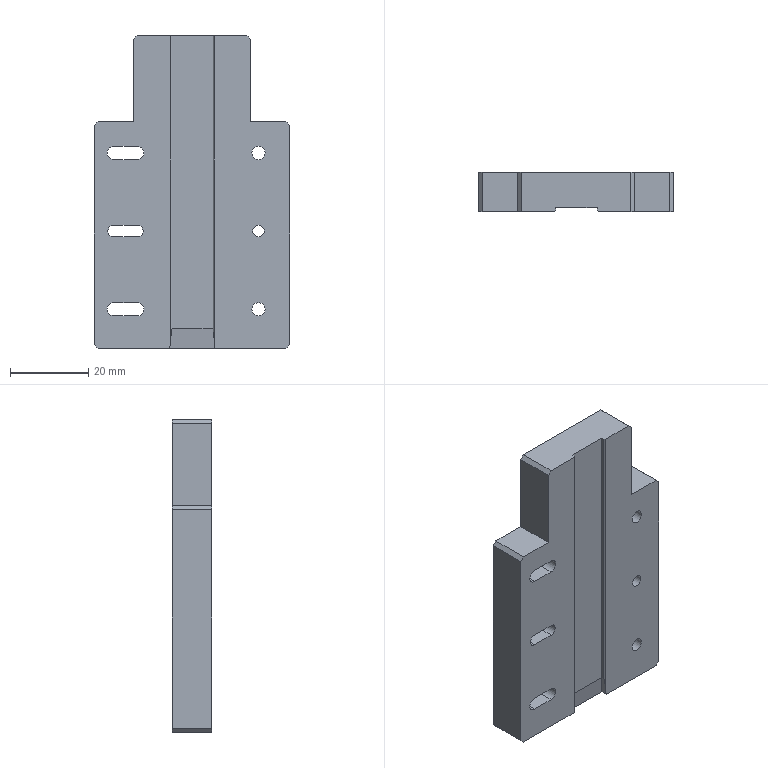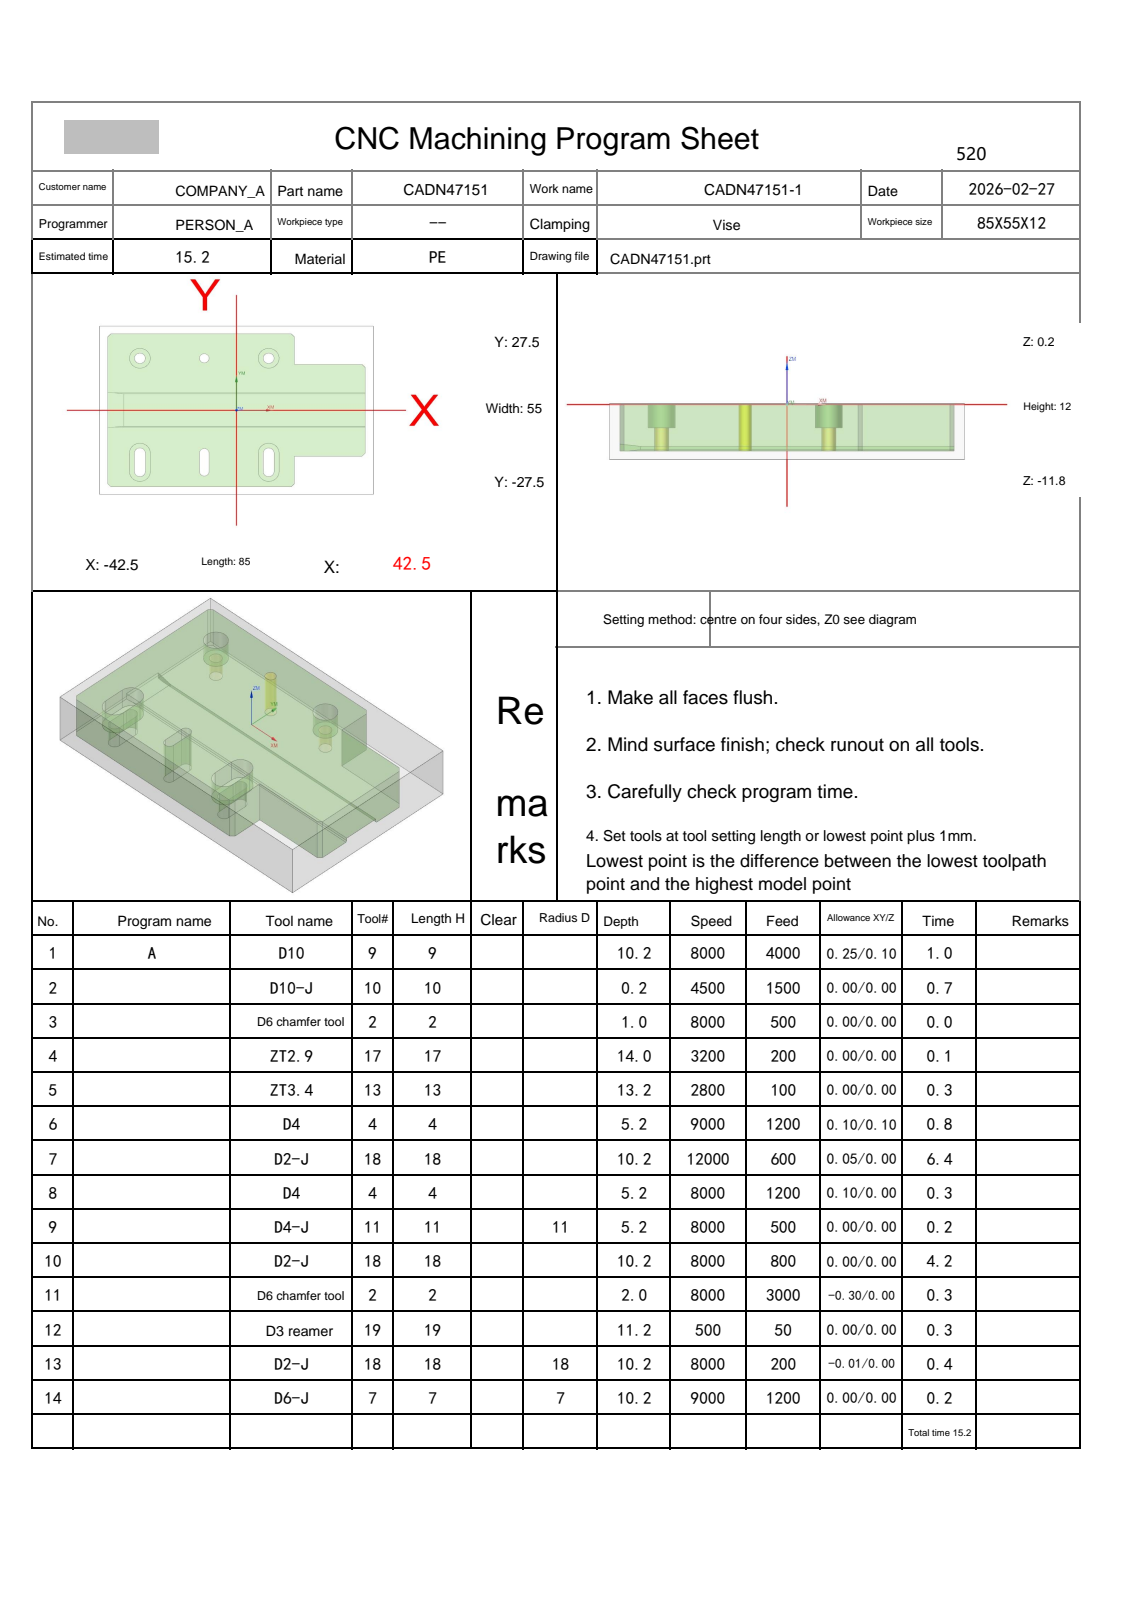NC program | NX | posted by the shop | part box 50 x 10 x 80 mm
Lines 7713 to 8100 of 8100:
N11 T02 M06
(D6 chamfer tool  D=6. R=0. H=02 ce=0.00 di=0.00)
G00 G90 G54 X-11.25 Y27.128 M03 S8000
G43 H02 Z50.
M08
Z2.099
G01 Z-1.5 F3000.
G03 X-11.33 Y26.828 I.52 J-.3
X-11.03 Y26.308 I.6 J0.0
G01 X-11. Y26.3
X17.
X17.254 Y26.275
X17.497 Y26.201
X17.722 Y26.081
X17.919 Y25.919
X18.919 Y24.919
X19.081 Y24.722
X19.201 Y24.497
X19.275 Y24.254
X19.3 Y24.
Y16.3
X39.
X39.254 Y16.275
X39.497 Y16.201
X39.722 Y16.081
X39.919 Y15.919
X40.919 Y14.919
X41.081 Y14.722
X41.201 Y14.497
X41.275 Y14.254
X41.3 Y14.
Y-14.
X41.275 Y-14.254
X41.201 Y-14.497
X41.081 Y-14.722
X40.919 Y-14.919
X39.919 Y-15.919
X39.722 Y-16.081
X39.497 Y-16.201
X39.254 Y-16.275
X39. Y-16.3
X19.3
Y-24.
X19.275 Y-24.254
X19.201 Y-24.497
X19.081 Y-24.722
X18.919 Y-24.919
X17.919 Y-25.919
X17.722 Y-26.081
X17.497 Y-26.201
X17.254 Y-26.275
X17. Y-26.3
X-39.
X-39.254 Y-26.275
X-39.497 Y-26.201
X-39.722 Y-26.081
X-39.919 Y-25.919
X-40.919 Y-24.919
X-41.081 Y-24.722
X-41.201 Y-24.497
X-41.275 Y-24.254
X-41.3 Y-24.
Y24.
X-41.275 Y24.254
X-41.201 Y24.497
X-41.081 Y24.722
X-40.919 Y24.919
X-39.919 Y25.919
X-39.722 Y26.081
X-39.497 Y26.201
X-39.254 Y26.275
X-39. Y26.3
X-11.
X-10.97 Y26.308
G03 X-10.67 Y26.828 I-.3 J.52
X-10.75 Y27.128 I-.6 J0.0
G01 Z2.099
G00 Z50.
X8.878 Y-16.75
Z2.099
G01 Z-1.5
G03 X8.578 Y-16.67 I-.3 J-.52
X8.058 Y-16.97 I0.0 J-.6
G01 X8.05 Y-17.
Y-20.
G03 X10. Y-21.95 I1.95 J0.0
X11.95 Y-20. I0.0 J1.95
G01 Y-14.
G03 X10. Y-12.05 I-1.95 J0.0
X8.05 Y-14. I0.0 J-1.95
G01 Y-17.
X8.058 Y-17.03
G03 X8.578 Y-17.33 I.52 J.3
X8.878 Y-17.25 I0.0 J.6
G01 Z2.099
G00 Z50.
X-9.786 Y-16.875
Z2.941
G01 Z-1.5
X-9.936 Y-16.835
G03 X-10.196 Y-16.985 I0.0 J-.3
G01 X-10.2 Y-17.
Y-20.
X-10.173 Y-20.1
X-10.1 Y-20.173
X-10. Y-20.2
X-9.9 Y-20.173
X-9.827 Y-20.1
X-9.8 Y-20.
Y-14.
X-9.827 Y-13.9
X-9.9 Y-13.827
X-10. Y-13.8
X-10.1 Y-13.827
X-10.173 Y-13.9
X-10.2 Y-14.
Y-17.
X-10.196 Y-17.015
G03 X-9.936 Y-17.165 I.26 J.15
G01 X-9.786 Y-17.125
Z2.941
G00 Z50.
X-28.878 Y-17.25
Z2.099
G01 Z-1.5
G03 X-28.578 Y-17.33 I.3 J.52
X-28.058 Y-17.03 I0.0 J.6
G01 X-28.05 Y-17.
Y-14.
G03 X-30. Y-12.05 I-1.95 J0.0
X-31.95 Y-14. I0.0 J-1.95
G01 Y-20.
G03 X-30. Y-21.95 I1.95 J0.0
X-28.05 Y-20. I0.0 J1.95
G01 Y-17.
X-28.058 Y-16.97
G03 X-28.578 Y-16.67 I-.52 J-.3
X-28.878 Y-16.75 I0.0 J-.6
G01 Z2.099
G00 Z50.
G00 G90 X-10. Y17. M03 S8000
Z50.
G98 G81 X-10. Y17. Z-1.8 R3. F500.
G80
G00 Z50.
G00 G90 X7.937 Y18.497 M03 S8000
Z50.
Z2.5
G01 X7.892 Y18.44 Z2.474 F500.
X7.719 Y18.147 Z2.35
X7.587 Y17.834 Z2.226
X7.498 Y17.507 Z2.103
X7.453 Y17.17 Z1.979
Y16.83 Z1.855
X7.498 Y16.493 Z1.732
X7.587 Y16.166 Z1.608
X7.719 Y15.853 Z1.484
X7.892 Y15.56 Z1.361
X8.102 Y15.293 Z1.237
X8.345 Y15.056 Z1.113
X8.618 Y14.854 Z.99
X8.832 Y14.73 Z.9
X9.144 Y14.595 Z.776
X9.471 Y14.502 Z.652
X9.807 Y14.454 Z.529
X10.147 Y14.451 Z.405
X10.484 Y14.493 Z.281
X10.812 Y14.58 Z.158
X11.127 Y14.709 Z.034
X11.421 Y14.879 Z-.089
X11.69 Y15.086 Z-.213
X11.929 Y15.328 Z-.337
X12.134 Y15.598 Z-.46
X12.301 Y15.894 Z-.584
X12.428 Y16.21 Z-.708
X12.511 Y16.539 Z-.831
X12.55 Y16.876 Z-.955
Y17. Z-1.
G03 X10. Y19.55 I-2.55 J0.0
X7.45 Y17. I0.0 J-2.55
X10. Y14.45 I2.55 J0.0
X12.55 Y17. I0.0 J2.55
X12.501 Y17.497 I-2.55 J0.0
G01 Z1.5
G00 Z50.
X-32.063 Y18.497
Z2.5
G01 X-32.108 Y18.44 Z2.474
X-32.281 Y18.147 Z2.35
X-32.413 Y17.834 Z2.226
X-32.502 Y17.507 Z2.103
X-32.547 Y17.17 Z1.979
Y16.83 Z1.855
X-32.502 Y16.493 Z1.732
X-32.413 Y16.166 Z1.608
X-32.281 Y15.853 Z1.484
X-32.108 Y15.56 Z1.361
X-31.898 Y15.293 Z1.237
X-31.655 Y15.056 Z1.113
X-31.382 Y14.854 Z.99
X-31.168 Y14.73 Z.9
X-30.856 Y14.595 Z.776
X-30.529 Y14.502 Z.652
X-30.193 Y14.454 Z.529
X-29.853 Y14.451 Z.405
X-29.516 Y14.493 Z.281
X-29.188 Y14.58 Z.158
X-28.873 Y14.709 Z.034
X-28.579 Y14.879 Z-.089
X-28.31 Y15.086 Z-.213
X-28.071 Y15.328 Z-.337
X-27.866 Y15.598 Z-.46
X-27.699 Y15.894 Z-.584
X-27.572 Y16.21 Z-.708
X-27.489 Y16.539 Z-.831
X-27.45 Y16.876 Z-.955
Y17. Z-1.
G03 X-30. Y19.55 I-2.55 J0.0
X-32.55 Y17. I0.0 J-2.55
X-30. Y14.45 I2.55 J0.0
X-27.45 Y17. I0.0 J2.55
X-27.499 Y17.497 I-2.55 J0.0
G01 Z1.5
G00 Z50.
G91 G28 Z0.0
M05
M09
G91 G28 Z0.0
M01
N12 T19 M06
(D3 reamer D=3. DR_a=180 H=19)
G00 G90 G54 X-10. Y17. M03 S500
G43 H19 Z50.
M08
G98 G81 X-10. Y17. Z-11. R1. F50.
G80
G00 Z50.
G91 G28 Z0.0
M05
M09
G91 G28 Z0.0
M01
N13 T18 M06
(D2-J  D=2. R=0. H=18 ce=-0.01 di=0.00)
G00 G90 G54 X-9.74 Y-17.2 M03 S8000
G43 H18 Z50.
M08
Z-1.5
G01 Z-2. F200.
G41 D18
X-9.69
G03 X-9.49 Y-17. I0.0 J.2
G01 Y-14.
G03 X-10. Y-13.49 I-.51 J0.0
X-10.51 Y-14. I0.0 J-.51
G01 Y-20.
G03 X-10. Y-20.51 I.51 J0.0
X-9.49 Y-20. I0.0 J.51
G01 Y-17.
Y-16.5
G03 X-9.69 Y-16.3 I-.2 J0.0
G01 G40 X-9.74
Z-1.5
G00 Z.5
Y-17.2
Z-3.5
G01 Z-4.
G41 D18
X-9.69
G03 X-9.49 Y-17. I0.0 J.2
G01 Y-14.
G03 X-10. Y-13.49 I-.51 J0.0
X-10.51 Y-14. I0.0 J-.51
G01 Y-20.
G03 X-10. Y-20.51 I.51 J0.0
X-9.49 Y-20. I0.0 J.51
G01 Y-17.
Y-16.5
G03 X-9.69 Y-16.3 I-.2 J0.0
G01 G40 X-9.74
Z-3.5
G00 Z-1.5
Y-17.2
Z-5.5
G01 Z-6.
G41 D18
X-9.69
G03 X-9.49 Y-17. I0.0 J.2
G01 Y-14.
G03 X-10. Y-13.49 I-.51 J0.0
X-10.51 Y-14. I0.0 J-.51
G01 Y-20.
G03 X-10. Y-20.51 I.51 J0.0
X-9.49 Y-20. I0.0 J.51
G01 Y-17.
Y-16.5
G03 X-9.69 Y-16.3 I-.2 J0.0
G01 G40 X-9.74
Z-5.5
G00 Z-3.5
Y-17.2
Z-7.5
G01 Z-8.
G41 D18
X-9.69
G03 X-9.49 Y-17. I0.0 J.2
G01 Y-14.
G03 X-10. Y-13.49 I-.51 J0.0
X-10.51 Y-14. I0.0 J-.51
G01 Y-20.
G03 X-10. Y-20.51 I.51 J0.0
X-9.49 Y-20. I0.0 J.51
G01 Y-17.
Y-16.5
G03 X-9.69 Y-16.3 I-.2 J0.0
G01 G40 X-9.74
Z-7.5
G00 Z-5.5
Y-17.2
Z-9.5
G01 Z-10.
G41 D18
X-9.69
G03 X-9.49 Y-17. I0.0 J.2
G01 Y-14.
G03 X-10. Y-13.49 I-.51 J0.0
X-10.51 Y-14. I0.0 J-.51
G01 Y-20.
G03 X-10. Y-20.51 I.51 J0.0
X-9.49 Y-20. I0.0 J.51
G01 Y-17.
Y-16.5
G03 X-9.69 Y-16.3 I-.2 J0.0
G01 G40 X-9.74
Z-9.5
G00 Z50.
G91 G28 Z0.0
M05
M09
G91 G28 Z0.0
M01
N14 T07 M06
(D6-J  D=6. R=0. H=07 ce=0.00 di=0.00)
G00 G90 G54 X18.017 Y-29.073 M03 S9000
G43 H07 Z50.
M08
Z-9.5
G01 Z-10. F1200.
G41 D07
X17.992 Y-28.875
G03 X17. Y-28. I-.992 J-.125
G01 X-39.
G02 X-41.121 Y-27.121 I0.0 J3.
G01 X-42.121 Y-26.121
G02 X-43. Y-24. I2.121 J2.121
G01 Y24.
G02 X-42.121 Y26.121 I3. J0.0
G01 X-41.121 Y27.121
G02 X-39. Y28. I2.121 J-2.121
G01 X17.
G02 X19.121 Y27.121 I0.0 J-3.
G01 X20.121 Y26.121
G02 X21. Y24. I-2.121 J-2.121
G01 Y18.
X39.
G02 X41.121 Y17.121 I0.0 J-3.
G01 X42.121 Y16.121
G02 X43. Y14. I-2.121 J-2.121
G01 Y-14.
G02 X42.121 Y-16.121 I-3. J0.0
G01 X41.121 Y-17.121
G02 X39. Y-18. I-2.121 J2.121
G01 X21.
Y-24.
G02 X20.121 Y-26.121 I-3. J0.0
G01 X19.121 Y-27.121
G02 X17. Y-28. I-2.121 J2.121
G01 X16.5
G03 X15.5 Y-29. I0.0 J-1.
G01 G40 Y-29.2
Z-9.5
G00 Z50.
M05
M09
G91 G28 Z0.0
G91 G28 Y0.0
M30
%